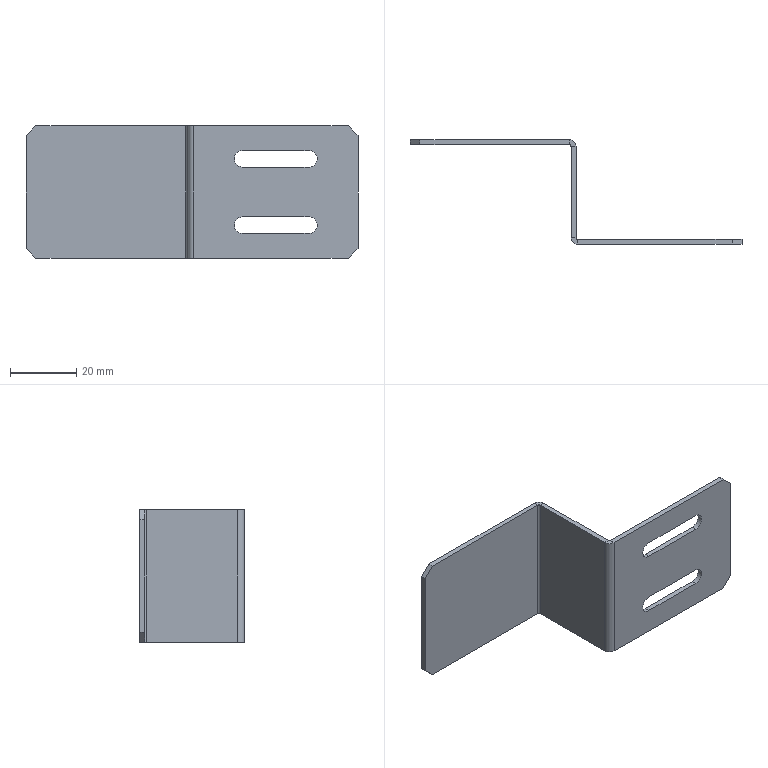Part | SolidWorks | features Chamfer 1, Cut 1, FlatPattern 1, SMBaseFlange 1, SheetMetal 1 | 1 solid | 34 faces | box 100 x 31.5 x 40 mm | volume 7350 mm3 | plane 26 | cylinder 8 | commonest cylinder face diameters 5 x4 1 x2 4 x2
STEP:
#1=CARTESIAN_POINT('',(0.,13.,20.));
#2=VERTEX_POINT('',#1);
#3=CARTESIAN_POINT('',(-1.5,13.,20.));
#4=VERTEX_POINT('',#3);
#5=CARTESIAN_POINT('',(0.,13.,20.));
#6=DIRECTION('',(-1.,0.,0.));
#7=VECTOR('',#6,1000.);
#8=LINE('',#5,#7);
#9=EDGE_CURVE('',#2,#4,#8,.T.);
#10=ORIENTED_EDGE('',*,*,#9,.F.);
#11=CARTESIAN_POINT('',(-2.,15.,20.));
#12=VERTEX_POINT('',#11);
#13=CARTESIAN_POINT('',(-2.,13.,20.));
#14=DIRECTION('',(0.,0.,-1.));
#15=DIRECTION('',(1.,0.,0.));
#16=AXIS2_PLACEMENT_3D('',#13,#14,#15);
#17=CIRCLE('',#16,2.);
#18=EDGE_CURVE('',#12,#2,#17,.T.);
#19=ORIENTED_EDGE('',*,*,#18,.F.);
#20=CARTESIAN_POINT('',(-2.,13.5,20.));
#21=VERTEX_POINT('',#20);
#22=CARTESIAN_POINT('',(-2.,13.5,20.));
#23=DIRECTION('',(0.,1.,0.));
#24=VECTOR('',#23,1000.);
#25=LINE('',#22,#24);
#26=EDGE_CURVE('',#21,#12,#25,.T.);
#27=ORIENTED_EDGE('',*,*,#26,.F.);
#28=CARTESIAN_POINT('',(-2.,13.,20.));
#29=DIRECTION('',(0.,0.,-1.));
#30=DIRECTION('',(1.,0.,0.));
#31=AXIS2_PLACEMENT_3D('',#28,#29,#30);
#32=CIRCLE('',#31,0.5);
#33=EDGE_CURVE('',#21,#4,#32,.T.);
#34=ORIENTED_EDGE('',*,*,#33,.T.);
#35=EDGE_LOOP('',(#10,#19,#27,#34));
#36=FACE_OUTER_BOUND('',#35,.T.);
#37=CARTESIAN_POINT('',(0.,13.,20.));
#38=DIRECTION('',(0.,0.,1.));
#39=DIRECTION('',(1.,0.,0.));
#40=AXIS2_PLACEMENT_3D('',#37,#38,#39);
#41=PLANE('',#40);
#42=ADVANCED_FACE('',(#36),#41,.T.);
#43=CARTESIAN_POINT('',(0.,-14.5,20.));
#44=VERTEX_POINT('',#43);
#45=CARTESIAN_POINT('',(0.,15.,20.));
#46=DIRECTION('',(0.,-1.,0.));
#47=VECTOR('',#46,1000.);
#48=LINE('',#45,#47);
#49=EDGE_CURVE('',#2,#44,#48,.T.);
#50=ORIENTED_EDGE('',*,*,#49,.F.);
#51=ORIENTED_EDGE('',*,*,#9,.T.);
#52=CARTESIAN_POINT('',(-1.5,-14.5,20.));
#53=VERTEX_POINT('',#52);
#54=CARTESIAN_POINT('',(-1.5,15.,20.));
#55=DIRECTION('',(0.,-1.,0.));
#56=VECTOR('',#55,1000.);
#57=LINE('',#54,#56);
#58=EDGE_CURVE('',#4,#53,#57,.T.);
#59=ORIENTED_EDGE('',*,*,#58,.T.);
#60=CARTESIAN_POINT('',(-1.5,-14.5,20.));
#61=DIRECTION('',(1.,0.,0.));
#62=VECTOR('',#61,1000.);
#63=LINE('',#60,#62);
#64=EDGE_CURVE('',#53,#44,#63,.T.);
#65=ORIENTED_EDGE('',*,*,#64,.T.);
#66=EDGE_LOOP('',(#50,#51,#59,#65));
#67=FACE_OUTER_BOUND('',#66,.T.);
#68=CARTESIAN_POINT('',(-2.,13.5,20.));
#69=DIRECTION('',(0.,0.,1.));
#70=DIRECTION('',(1.,0.,0.));
#71=AXIS2_PLACEMENT_3D('',#68,#69,#70);
#72=PLANE('',#71);
#73=ADVANCED_FACE('',(#67),#72,.T.);
#74=CARTESIAN_POINT('',(-2.,15.,-20.));
#75=VERTEX_POINT('',#74);
#76=CARTESIAN_POINT('',(-2.,13.5,-20.));
#77=VERTEX_POINT('',#76);
#78=CARTESIAN_POINT('',(-2.,15.,-20.));
#79=DIRECTION('',(0.,-1.,0.));
#80=VECTOR('',#79,1000.);
#81=LINE('',#78,#80);
#82=EDGE_CURVE('',#75,#77,#81,.T.);
#83=ORIENTED_EDGE('',*,*,#82,.F.);
#84=CARTESIAN_POINT('',(0.,13.,-20.));
#85=VERTEX_POINT('',#84);
#86=CARTESIAN_POINT('',(-2.,13.,-20.));
#87=DIRECTION('',(0.,0.,-1.));
#88=DIRECTION('',(1.,0.,0.));
#89=AXIS2_PLACEMENT_3D('',#86,#87,#88);
#90=CIRCLE('',#89,2.);
#91=EDGE_CURVE('',#75,#85,#90,.T.);
#92=ORIENTED_EDGE('',*,*,#91,.T.);
#93=CARTESIAN_POINT('',(-1.5,13.,-20.));
#94=VERTEX_POINT('',#93);
#95=CARTESIAN_POINT('',(-1.5,13.,-20.));
#96=DIRECTION('',(1.,0.,0.));
#97=VECTOR('',#96,1000.);
#98=LINE('',#95,#97);
#99=EDGE_CURVE('',#94,#85,#98,.T.);
#100=ORIENTED_EDGE('',*,*,#99,.F.);
#101=CARTESIAN_POINT('',(-2.,13.,-20.));
#102=DIRECTION('',(0.,0.,-1.));
#103=DIRECTION('',(1.,0.,0.));
#104=AXIS2_PLACEMENT_3D('',#101,#102,#103);
#105=CIRCLE('',#104,0.5);
#106=EDGE_CURVE('',#77,#94,#105,.T.);
#107=ORIENTED_EDGE('',*,*,#106,.F.);
#108=EDGE_LOOP('',(#83,#92,#100,#107));
#109=FACE_OUTER_BOUND('',#108,.T.);
#110=CARTESIAN_POINT('',(-2.,15.,-20.));
#111=DIRECTION('',(0.,0.,-1.));
#112=DIRECTION('',(-1.,0.,0.));
#113=AXIS2_PLACEMENT_3D('',#110,#111,#112);
#114=PLANE('',#113);
#115=ADVANCED_FACE('',(#109),#114,.T.);
#116=CARTESIAN_POINT('',(-47.,13.5,-20.));
#117=VERTEX_POINT('',#116);
#118=CARTESIAN_POINT('',(-50.,13.5,-20.));
#119=DIRECTION('',(1.,0.,0.));
#120=VECTOR('',#119,1000.);
#121=LINE('',#118,#120);
#122=EDGE_CURVE('',#117,#77,#121,.T.);
#123=ORIENTED_EDGE('',*,*,#122,.F.);
#124=CARTESIAN_POINT('',(-47.,15.,-20.));
#125=VERTEX_POINT('',#124);
#126=CARTESIAN_POINT('',(-47.,13.,-20.));
#127=DIRECTION('',(0.,1.,0.));
#128=VECTOR('',#127,1000.);
#129=LINE('',#126,#128);
#130=EDGE_CURVE('',#117,#125,#129,.T.);
#131=ORIENTED_EDGE('',*,*,#130,.T.);
#132=CARTESIAN_POINT('',(-50.,15.,-20.));
#133=DIRECTION('',(1.,0.,0.));
#134=VECTOR('',#133,1000.);
#135=LINE('',#132,#134);
#136=EDGE_CURVE('',#125,#75,#135,.T.);
#137=ORIENTED_EDGE('',*,*,#136,.T.);
#138=ORIENTED_EDGE('',*,*,#82,.T.);
#139=EDGE_LOOP('',(#123,#131,#137,#138));
#140=FACE_OUTER_BOUND('',#139,.T.);
#141=CARTESIAN_POINT('',(-1.5,13.,-20.));
#142=DIRECTION('',(0.,0.,-1.));
#143=DIRECTION('',(-1.,0.,0.));
#144=AXIS2_PLACEMENT_3D('',#141,#142,#143);
#145=PLANE('',#144);
#146=ADVANCED_FACE('',(#140),#145,.T.);
#147=CARTESIAN_POINT('',(0.5,-15.,20.));
#148=VERTEX_POINT('',#147);
#149=CARTESIAN_POINT('',(0.5,-16.5,20.));
#150=VERTEX_POINT('',#149);
#151=CARTESIAN_POINT('',(0.5,-15.,20.));
#152=DIRECTION('',(0.,-1.,0.));
#153=VECTOR('',#152,1000.);
#154=LINE('',#151,#153);
#155=EDGE_CURVE('',#148,#150,#154,.T.);
#156=ORIENTED_EDGE('',*,*,#155,.F.);
#157=CARTESIAN_POINT('',(0.5,-14.5,20.));
#158=DIRECTION('',(0.,0.,1.));
#159=DIRECTION('',(-1.,0.,0.));
#160=AXIS2_PLACEMENT_3D('',#157,#158,#159);
#161=CIRCLE('',#160,0.5);
#162=EDGE_CURVE('',#44,#148,#161,.T.);
#163=ORIENTED_EDGE('',*,*,#162,.F.);
#164=ORIENTED_EDGE('',*,*,#64,.F.);
#165=CARTESIAN_POINT('',(0.5,-14.5,20.));
#166=DIRECTION('',(0.,0.,1.));
#167=DIRECTION('',(1.,0.,0.));
#168=AXIS2_PLACEMENT_3D('',#165,#166,#167);
#169=CIRCLE('',#168,2.);
#170=EDGE_CURVE('',#53,#150,#169,.T.);
#171=ORIENTED_EDGE('',*,*,#170,.T.);
#172=EDGE_LOOP('',(#156,#163,#164,#171));
#173=FACE_OUTER_BOUND('',#172,.T.);
#174=CARTESIAN_POINT('',(0.5,-15.,20.));
#175=DIRECTION('',(0.,0.,1.));
#176=DIRECTION('',(1.,0.,0.));
#177=AXIS2_PLACEMENT_3D('',#174,#175,#176);
#178=PLANE('',#177);
#179=ADVANCED_FACE('',(#173),#178,.T.);
#180=CARTESIAN_POINT('',(47.,-16.5,20.));
#181=VERTEX_POINT('',#180);
#182=CARTESIAN_POINT('',(0.,-16.5,20.));
#183=DIRECTION('',(1.,0.,0.));
#184=VECTOR('',#183,1000.);
#185=LINE('',#182,#184);
#186=EDGE_CURVE('',#150,#181,#185,.T.);
#187=ORIENTED_EDGE('',*,*,#186,.T.);
#188=CARTESIAN_POINT('',(47.,-15.,20.));
#189=VERTEX_POINT('',#188);
#190=CARTESIAN_POINT('',(47.,-14.5,20.));
#191=DIRECTION('',(0.,1.,0.));
#192=VECTOR('',#191,1000.);
#193=LINE('',#190,#192);
#194=EDGE_CURVE('',#181,#189,#193,.T.);
#195=ORIENTED_EDGE('',*,*,#194,.T.);
#196=CARTESIAN_POINT('',(0.,-15.,20.));
#197=DIRECTION('',(1.,0.,0.));
#198=VECTOR('',#197,1000.);
#199=LINE('',#196,#198);
#200=EDGE_CURVE('',#148,#189,#199,.T.);
#201=ORIENTED_EDGE('',*,*,#200,.F.);
#202=ORIENTED_EDGE('',*,*,#155,.T.);
#203=EDGE_LOOP('',(#187,#195,#201,#202));
#204=FACE_OUTER_BOUND('',#203,.T.);
#205=CARTESIAN_POINT('',(-1.5,-14.5,20.));
#206=DIRECTION('',(0.,0.,1.));
#207=DIRECTION('',(1.,0.,0.));
#208=AXIS2_PLACEMENT_3D('',#205,#206,#207);
#209=PLANE('',#208);
#210=ADVANCED_FACE('',(#204),#209,.T.);
#211=CARTESIAN_POINT('',(0.,-14.5,-20.));
#212=VERTEX_POINT('',#211);
#213=CARTESIAN_POINT('',(-1.5,-14.5,-20.));
#214=VERTEX_POINT('',#213);
#215=CARTESIAN_POINT('',(0.,-14.5,-20.));
#216=DIRECTION('',(-1.,0.,0.));
#217=VECTOR('',#216,1000.);
#218=LINE('',#215,#217);
#219=EDGE_CURVE('',#212,#214,#218,.T.);
#220=ORIENTED_EDGE('',*,*,#219,.F.);
#221=CARTESIAN_POINT('',(0.5,-15.,-20.));
#222=VERTEX_POINT('',#221);
#223=CARTESIAN_POINT('',(0.5,-14.5,-20.));
#224=DIRECTION('',(0.,0.,1.));
#225=DIRECTION('',(-1.,0.,0.));
#226=AXIS2_PLACEMENT_3D('',#223,#224,#225);
#227=CIRCLE('',#226,0.5);
#228=EDGE_CURVE('',#212,#222,#227,.T.);
#229=ORIENTED_EDGE('',*,*,#228,.T.);
#230=CARTESIAN_POINT('',(0.5,-16.5,-20.));
#231=VERTEX_POINT('',#230);
#232=CARTESIAN_POINT('',(0.5,-16.5,-20.));
#233=DIRECTION('',(0.,1.,0.));
#234=VECTOR('',#233,1000.);
#235=LINE('',#232,#234);
#236=EDGE_CURVE('',#231,#222,#235,.T.);
#237=ORIENTED_EDGE('',*,*,#236,.F.);
#238=CARTESIAN_POINT('',(0.5,-14.5,-20.));
#239=DIRECTION('',(0.,0.,1.));
#240=DIRECTION('',(1.,0.,0.));
#241=AXIS2_PLACEMENT_3D('',#238,#239,#240);
#242=CIRCLE('',#241,2.);
#243=EDGE_CURVE('',#214,#231,#242,.T.);
#244=ORIENTED_EDGE('',*,*,#243,.F.);
#245=EDGE_LOOP('',(#220,#229,#237,#244));
#246=FACE_OUTER_BOUND('',#245,.T.);
#247=CARTESIAN_POINT('',(0.,-14.5,-20.));
#248=DIRECTION('',(0.,0.,-1.));
#249=DIRECTION('',(-1.,0.,0.));
#250=AXIS2_PLACEMENT_3D('',#247,#248,#249);
#251=PLANE('',#250);
#252=ADVANCED_FACE('',(#246),#251,.T.);
#253=CARTESIAN_POINT('',(0.,15.,-20.));
#254=DIRECTION('',(0.,-1.,0.));
#255=VECTOR('',#254,1000.);
#256=LINE('',#253,#255);
#257=EDGE_CURVE('',#85,#212,#256,.T.);
#258=ORIENTED_EDGE('',*,*,#257,.T.);
#259=ORIENTED_EDGE('',*,*,#219,.T.);
#260=CARTESIAN_POINT('',(-1.5,15.,-20.));
#261=DIRECTION('',(0.,-1.,0.));
#262=VECTOR('',#261,1000.);
#263=LINE('',#260,#262);
#264=EDGE_CURVE('',#94,#214,#263,.T.);
#265=ORIENTED_EDGE('',*,*,#264,.F.);
#266=ORIENTED_EDGE('',*,*,#99,.T.);
#267=EDGE_LOOP('',(#258,#259,#265,#266));
#268=FACE_OUTER_BOUND('',#267,.T.);
#269=CARTESIAN_POINT('',(0.5,-16.5,-20.));
#270=DIRECTION('',(0.,0.,-1.));
#271=DIRECTION('',(-1.,0.,0.));
#272=AXIS2_PLACEMENT_3D('',#269,#270,#271);
#273=PLANE('',#272);
#274=ADVANCED_FACE('',(#268),#273,.T.);
#275=CARTESIAN_POINT('',(35.25,-16.5,-12.5));
#276=VERTEX_POINT('',#275);
#277=CARTESIAN_POINT('',(15.25,-16.5,-12.5));
#278=VERTEX_POINT('',#277);
#279=CARTESIAN_POINT('',(15.25,-16.5,-12.5));
#280=DIRECTION('',(-1.,0.,0.));
#281=VECTOR('',#280,1000.);
#282=LINE('',#279,#281);
#283=EDGE_CURVE('',#276,#278,#282,.T.);
#284=ORIENTED_EDGE('',*,*,#283,.T.);
#285=CARTESIAN_POINT('',(15.25,-16.5,-7.5));
#286=VERTEX_POINT('',#285);
#287=CARTESIAN_POINT('',(15.25,-16.5,-10.));
#288=DIRECTION('',(0.,1.,0.));
#289=DIRECTION('',(0.,0.,1.));
#290=AXIS2_PLACEMENT_3D('',#287,#288,#289);
#291=CIRCLE('',#290,2.5);
#292=EDGE_CURVE('',#278,#286,#291,.T.);
#293=ORIENTED_EDGE('',*,*,#292,.T.);
#294=CARTESIAN_POINT('',(35.25,-16.5,-7.5));
#295=VERTEX_POINT('',#294);
#296=CARTESIAN_POINT('',(15.25,-16.5,-7.5));
#297=DIRECTION('',(1.,0.,0.));
#298=VECTOR('',#297,1000.);
#299=LINE('',#296,#298);
#300=EDGE_CURVE('',#286,#295,#299,.T.);
#301=ORIENTED_EDGE('',*,*,#300,.T.);
#302=CARTESIAN_POINT('',(35.25,-16.5,-10.));
#303=DIRECTION('',(0.,1.,0.));
#304=DIRECTION('',(0.,0.,1.));
#305=AXIS2_PLACEMENT_3D('',#302,#303,#304);
#306=CIRCLE('',#305,2.5);
#307=EDGE_CURVE('',#295,#276,#306,.T.);
#308=ORIENTED_EDGE('',*,*,#307,.T.);
#309=EDGE_LOOP('',(#284,#293,#301,#308));
#310=FACE_BOUND('',#309,.T.);
#311=CARTESIAN_POINT('',(35.25,-16.5,7.5));
#312=VERTEX_POINT('',#311);
#313=CARTESIAN_POINT('',(15.25,-16.5,7.5));
#314=VERTEX_POINT('',#313);
#315=CARTESIAN_POINT('',(15.25,-16.5,7.5));
#316=DIRECTION('',(-1.,0.,0.));
#317=VECTOR('',#316,1000.);
#318=LINE('',#315,#317);
#319=EDGE_CURVE('',#312,#314,#318,.T.);
#320=ORIENTED_EDGE('',*,*,#319,.T.);
#321=CARTESIAN_POINT('',(15.25,-16.5,12.5));
#322=VERTEX_POINT('',#321);
#323=CARTESIAN_POINT('',(15.25,-16.5,10.));
#324=DIRECTION('',(0.,1.,0.));
#325=DIRECTION('',(0.,0.,1.));
#326=AXIS2_PLACEMENT_3D('',#323,#324,#325);
#327=CIRCLE('',#326,2.5);
#328=EDGE_CURVE('',#314,#322,#327,.T.);
#329=ORIENTED_EDGE('',*,*,#328,.T.);
#330=CARTESIAN_POINT('',(35.25,-16.5,12.5));
#331=VERTEX_POINT('',#330);
#332=CARTESIAN_POINT('',(15.25,-16.5,12.5));
#333=DIRECTION('',(1.,0.,0.));
#334=VECTOR('',#333,1000.);
#335=LINE('',#332,#334);
#336=EDGE_CURVE('',#322,#331,#335,.T.);
#337=ORIENTED_EDGE('',*,*,#336,.T.);
#338=CARTESIAN_POINT('',(35.25,-16.5,10.));
#339=DIRECTION('',(0.,1.,0.));
#340=DIRECTION('',(0.,0.,1.));
#341=AXIS2_PLACEMENT_3D('',#338,#339,#340);
#342=CIRCLE('',#341,2.5);
#343=EDGE_CURVE('',#331,#312,#342,.T.);
#344=ORIENTED_EDGE('',*,*,#343,.T.);
#345=EDGE_LOOP('',(#320,#329,#337,#344));
#346=FACE_BOUND('',#345,.T.);
#347=CARTESIAN_POINT('',(47.,-16.5,-20.));
#348=VERTEX_POINT('',#347);
#349=CARTESIAN_POINT('',(0.,-16.5,-20.));
#350=DIRECTION('',(1.,0.,0.));
#351=VECTOR('',#350,1000.);
#352=LINE('',#349,#351);
#353=EDGE_CURVE('',#231,#348,#352,.T.);
#354=ORIENTED_EDGE('',*,*,#353,.T.);
#355=CARTESIAN_POINT('',(50.,-16.5,-17.));
#356=VERTEX_POINT('',#355);
#357=CARTESIAN_POINT('',(47.,-16.5,-20.));
#358=DIRECTION('',(0.7071,0.,0.7071));
#359=VECTOR('',#358,1000.);
#360=LINE('',#357,#359);
#361=EDGE_CURVE('',#348,#356,#360,.T.);
#362=ORIENTED_EDGE('',*,*,#361,.T.);
#363=CARTESIAN_POINT('',(50.,-16.5,17.));
#364=VERTEX_POINT('',#363);
#365=CARTESIAN_POINT('',(50.,-16.5,20.));
#366=DIRECTION('',(0.,0.,-1.));
#367=VECTOR('',#366,1000.);
#368=LINE('',#365,#367);
#369=EDGE_CURVE('',#364,#356,#368,.T.);
#370=ORIENTED_EDGE('',*,*,#369,.F.);
#371=CARTESIAN_POINT('',(50.,-16.5,17.));
#372=DIRECTION('',(-0.7071,0.,0.7071));
#373=VECTOR('',#372,1000.);
#374=LINE('',#371,#373);
#375=EDGE_CURVE('',#364,#181,#374,.T.);
#376=ORIENTED_EDGE('',*,*,#375,.T.);
#377=ORIENTED_EDGE('',*,*,#186,.F.);
#378=CARTESIAN_POINT('',(0.5,-16.5,20.));
#379=DIRECTION('',(0.,0.,-1.));
#380=VECTOR('',#379,1000.);
#381=LINE('',#378,#380);
#382=EDGE_CURVE('',#150,#231,#381,.T.);
#383=ORIENTED_EDGE('',*,*,#382,.T.);
#384=EDGE_LOOP('',(#354,#362,#370,#376,#377,#383));
#385=FACE_OUTER_BOUND('',#384,.T.);
#386=CARTESIAN_POINT('',(0.,-16.5,20.));
#387=DIRECTION('',(0.,1.,0.));
#388=DIRECTION('',(0.,0.,1.));
#389=AXIS2_PLACEMENT_3D('',#386,#387,#388);
#390=PLANE('',#389);
#391=ADVANCED_FACE('',(#310,#346,#385),#390,.F.);
#392=ORIENTED_EDGE('',*,*,#369,.T.);
#393=CARTESIAN_POINT('',(50.,-15.,-17.));
#394=VERTEX_POINT('',#393);
#395=CARTESIAN_POINT('',(50.,-15.,-17.));
#396=DIRECTION('',(0.,1.,0.));
#397=VECTOR('',#396,1000.);
#398=LINE('',#395,#397);
#399=EDGE_CURVE('',#356,#394,#398,.T.);
#400=ORIENTED_EDGE('',*,*,#399,.T.);
#401=CARTESIAN_POINT('',(50.,-15.,17.));
#402=VERTEX_POINT('',#401);
#403=CARTESIAN_POINT('',(50.,-15.,20.));
#404=DIRECTION('',(0.,0.,-1.));
#405=VECTOR('',#404,1000.);
#406=LINE('',#403,#405);
#407=EDGE_CURVE('',#402,#394,#406,.T.);
#408=ORIENTED_EDGE('',*,*,#407,.F.);
#409=CARTESIAN_POINT('',(50.,-15.,17.));
#410=DIRECTION('',(0.,-1.,0.));
#411=VECTOR('',#410,1000.);
#412=LINE('',#409,#411);
#413=EDGE_CURVE('',#402,#364,#412,.T.);
#414=ORIENTED_EDGE('',*,*,#413,.T.);
#415=EDGE_LOOP('',(#392,#400,#408,#414));
#416=FACE_OUTER_BOUND('',#415,.T.);
#417=CARTESIAN_POINT('',(50.,-15.,20.));
#418=DIRECTION('',(1.,0.,0.));
#419=DIRECTION('',(0.,0.,-1.));
#420=AXIS2_PLACEMENT_3D('',#417,#418,#419);
#421=PLANE('',#420);
#422=ADVANCED_FACE('',(#416),#421,.T.);
#423=CARTESIAN_POINT('',(15.25,-15.,-12.5));
#424=VERTEX_POINT('',#423);
#425=CARTESIAN_POINT('',(15.25,-15.,-7.5));
#426=VERTEX_POINT('',#425);
#427=CARTESIAN_POINT('',(15.25,-15.,-10.));
#428=DIRECTION('',(0.,1.,0.));
#429=DIRECTION('',(0.,0.,1.));
#430=AXIS2_PLACEMENT_3D('',#427,#428,#429);
#431=CIRCLE('',#430,2.5);
#432=EDGE_CURVE('',#424,#426,#431,.T.);
#433=ORIENTED_EDGE('',*,*,#432,.F.);
#434=CARTESIAN_POINT('',(35.25,-15.,-12.5));
#435=VERTEX_POINT('',#434);
#436=CARTESIAN_POINT('',(15.25,-15.,-12.5));
#437=DIRECTION('',(-1.,0.,0.));
#438=VECTOR('',#437,1000.);
#439=LINE('',#436,#438);
#440=EDGE_CURVE('',#435,#424,#439,.T.);
#441=ORIENTED_EDGE('',*,*,#440,.F.);
#442=CARTESIAN_POINT('',(35.25,-15.,-7.5));
#443=VERTEX_POINT('',#442);
#444=CARTESIAN_POINT('',(35.25,-15.,-10.));
#445=DIRECTION('',(0.,1.,0.));
#446=DIRECTION('',(0.,0.,1.));
#447=AXIS2_PLACEMENT_3D('',#444,#445,#446);
#448=CIRCLE('',#447,2.5);
#449=EDGE_CURVE('',#443,#435,#448,.T.);
#450=ORIENTED_EDGE('',*,*,#449,.F.);
#451=CARTESIAN_POINT('',(15.25,-15.,-7.5));
#452=DIRECTION('',(1.,0.,0.));
#453=VECTOR('',#452,1000.);
#454=LINE('',#451,#453);
#455=EDGE_CURVE('',#426,#443,#454,.T.);
#456=ORIENTED_EDGE('',*,*,#455,.F.);
#457=EDGE_LOOP('',(#433,#441,#450,#456));
#458=FACE_BOUND('',#457,.T.);
#459=CARTESIAN_POINT('',(15.25,-15.,7.5));
#460=VERTEX_POINT('',#459);
#461=CARTESIAN_POINT('',(15.25,-15.,12.5));
#462=VERTEX_POINT('',#461);
#463=CARTESIAN_POINT('',(15.25,-15.,10.));
#464=DIRECTION('',(0.,1.,0.));
#465=DIRECTION('',(0.,0.,1.));
#466=AXIS2_PLACEMENT_3D('',#463,#464,#465);
#467=CIRCLE('',#466,2.5);
#468=EDGE_CURVE('',#460,#462,#467,.T.);
#469=ORIENTED_EDGE('',*,*,#468,.F.);
#470=CARTESIAN_POINT('',(35.25,-15.,7.5));
#471=VERTEX_POINT('',#470);
#472=CARTESIAN_POINT('',(15.25,-15.,7.5));
#473=DIRECTION('',(-1.,0.,0.));
#474=VECTOR('',#473,1000.);
#475=LINE('',#472,#474);
#476=EDGE_CURVE('',#471,#460,#475,.T.);
#477=ORIENTED_EDGE('',*,*,#476,.F.);
#478=CARTESIAN_POINT('',(35.25,-15.,12.5));
#479=VERTEX_POINT('',#478);
#480=CARTESIAN_POINT('',(35.25,-15.,10.));
#481=DIRECTION('',(0.,1.,0.));
#482=DIRECTION('',(0.,0.,1.));
#483=AXIS2_PLACEMENT_3D('',#480,#481,#482);
#484=CIRCLE('',#483,2.5);
#485=EDGE_CURVE('',#479,#471,#484,.T.);
#486=ORIENTED_EDGE('',*,*,#485,.F.);
#487=CARTESIAN_POINT('',(15.25,-15.,12.5));
#488=DIRECTION('',(1.,0.,0.));
#489=VECTOR('',#488,1000.);
#490=LINE('',#487,#489);
#491=EDGE_CURVE('',#462,#479,#490,.T.);
#492=ORIENTED_EDGE('',*,*,#491,.F.);
#493=EDGE_LOOP('',(#469,#477,#486,#492));
#494=FACE_BOUND('',#493,.T.);
#495=ORIENTED_EDGE('',*,*,#407,.T.);
#496=CARTESIAN_POINT('',(47.,-15.,-20.));
#497=VERTEX_POINT('',#496);
#498=CARTESIAN_POINT('',(43.5,-15.,-23.5));
#499=DIRECTION('',(-0.7071,0.,-0.7071));
#500=VECTOR('',#499,1000.);
#501=LINE('',#498,#500);
#502=EDGE_CURVE('',#394,#497,#501,.T.);
#503=ORIENTED_EDGE('',*,*,#502,.T.);
#504=CARTESIAN_POINT('',(0.,-15.,-20.));
#505=DIRECTION('',(1.,0.,0.));
#506=VECTOR('',#505,1000.);
#507=LINE('',#504,#506);
#508=EDGE_CURVE('',#222,#497,#507,.T.);
#509=ORIENTED_EDGE('',*,*,#508,.F.);
#510=CARTESIAN_POINT('',(0.5,-15.,20.));
#511=DIRECTION('',(0.,0.,-1.));
#512=VECTOR('',#511,1000.);
#513=LINE('',#510,#512);
#514=EDGE_CURVE('',#148,#222,#513,.T.);
#515=ORIENTED_EDGE('',*,*,#514,.F.);
#516=ORIENTED_EDGE('',*,*,#200,.T.);
#517=CARTESIAN_POINT('',(23.5,-15.,43.5));
#518=DIRECTION('',(0.7071,0.,-0.7071));
#519=VECTOR('',#518,1000.);
#520=LINE('',#517,#519);
#521=EDGE_CURVE('',#189,#402,#520,.T.);
#522=ORIENTED_EDGE('',*,*,#521,.T.);
#523=EDGE_LOOP('',(#495,#503,#509,#515,#516,#522));
#524=FACE_OUTER_BOUND('',#523,.T.);
#525=CARTESIAN_POINT('',(0.,-15.,20.));
#526=DIRECTION('',(0.,1.,0.));
#527=DIRECTION('',(0.,0.,1.));
#528=AXIS2_PLACEMENT_3D('',#525,#526,#527);
#529=PLANE('',#528);
#530=ADVANCED_FACE('',(#458,#494,#524),#529,.T.);
#531=ORIENTED_EDGE('',*,*,#228,.F.);
#532=CARTESIAN_POINT('',(0.,-14.5,20.));
#533=DIRECTION('',(0.,0.,-1.));
#534=VECTOR('',#533,1000.);
#535=LINE('',#532,#534);
#536=EDGE_CURVE('',#44,#212,#535,.T.);
#537=ORIENTED_EDGE('',*,*,#536,.F.);
#538=ORIENTED_EDGE('',*,*,#162,.T.);
#539=ORIENTED_EDGE('',*,*,#514,.T.);
#540=EDGE_LOOP('',(#531,#537,#538,#539));
#541=FACE_OUTER_BOUND('',#540,.T.);
#542=CARTESIAN_POINT('',(0.5,-14.5,20.));
#543=DIRECTION('',(0.,0.,-1.));
#544=DIRECTION('',(-1.,0.,0.));
#545=AXIS2_PLACEMENT_3D('',#542,#543,#544);
#546=CYLINDRICAL_SURFACE('',#545,0.5);
#547=ADVANCED_FACE('',(#541),#546,.F.);
#548=ORIENTED_EDGE('',*,*,#257,.F.);
#549=CARTESIAN_POINT('',(0.,13.,20.));
#550=DIRECTION('',(0.,0.,-1.));
#551=VECTOR('',#550,1000.);
#552=LINE('',#549,#551);
#553=EDGE_CURVE('',#2,#85,#552,.T.);
#554=ORIENTED_EDGE('',*,*,#553,.F.);
#555=ORIENTED_EDGE('',*,*,#49,.T.);
#556=ORIENTED_EDGE('',*,*,#536,.T.);
#557=EDGE_LOOP('',(#548,#554,#555,#556));
#558=FACE_OUTER_BOUND('',#557,.T.);
#559=CARTESIAN_POINT('',(0.,15.,20.));
#560=DIRECTION('',(1.,0.,0.));
#561=DIRECTION('',(0.,0.,-1.));
#562=AXIS2_PLACEMENT_3D('',#559,#560,#561);
#563=PLANE('',#562);
#564=ADVANCED_FACE('',(#558),#563,.T.);
#565=ORIENTED_EDGE('',*,*,#91,.F.);
#566=CARTESIAN_POINT('',(-2.,15.,20.));
#567=DIRECTION('',(0.,0.,-1.));
#568=VECTOR('',#567,1000.);
#569=LINE('',#566,#568);
#570=EDGE_CURVE('',#12,#75,#569,.T.);
#571=ORIENTED_EDGE('',*,*,#570,.F.);
#572=ORIENTED_EDGE('',*,*,#18,.T.);
#573=ORIENTED_EDGE('',*,*,#553,.T.);
#574=EDGE_LOOP('',(#565,#571,#572,#573));
#575=FACE_OUTER_BOUND('',#574,.T.);
#576=CARTESIAN_POINT('',(-2.,13.,20.));
#577=DIRECTION('',(0.,0.,-1.));
#578=DIRECTION('',(-1.,0.,0.));
#579=AXIS2_PLACEMENT_3D('',#576,#577,#578);
#580=CYLINDRICAL_SURFACE('',#579,2.);
#581=ADVANCED_FACE('',(#575),#580,.T.);
#582=ORIENTED_EDGE('',*,*,#136,.F.);
#583=CARTESIAN_POINT('',(-50.,15.,-17.));
#584=VERTEX_POINT('',#583);
#585=CARTESIAN_POINT('',(-68.5,15.,1.5));
#586=DIRECTION('',(-0.7071,0.,0.7071));
#587=VECTOR('',#586,1000.);
#588=LINE('',#585,#587);
#589=EDGE_CURVE('',#125,#584,#588,.T.);
#590=ORIENTED_EDGE('',*,*,#589,.T.);
#591=CARTESIAN_POINT('',(-50.,15.,17.));
#592=VERTEX_POINT('',#591);
#593=CARTESIAN_POINT('',(-50.,15.,20.));
#594=DIRECTION('',(0.,0.,-1.));
#595=VECTOR('',#594,1000.);
#596=LINE('',#593,#595);
#597=EDGE_CURVE('',#592,#584,#596,.T.);
#598=ORIENTED_EDGE('',*,*,#597,.F.);
#599=CARTESIAN_POINT('',(-47.,15.,20.));
#600=VERTEX_POINT('',#599);
#601=CARTESIAN_POINT('',(-48.5,15.,18.5));
#602=DIRECTION('',(0.7071,0.,0.7071));
#603=VECTOR('',#602,1000.);
#604=LINE('',#601,#603);
#605=EDGE_CURVE('',#592,#600,#604,.T.);
#606=ORIENTED_EDGE('',*,*,#605,.T.);
#607=CARTESIAN_POINT('',(-50.,15.,20.));
#608=DIRECTION('',(1.,0.,0.));
#609=VECTOR('',#608,1000.);
#610=LINE('',#607,#609);
#611=EDGE_CURVE('',#600,#12,#610,.T.);
#612=ORIENTED_EDGE('',*,*,#611,.T.);
#613=ORIENTED_EDGE('',*,*,#570,.T.);
#614=EDGE_LOOP('',(#582,#590,#598,#606,#612,#613));
#615=FACE_OUTER_BOUND('',#614,.T.);
#616=CARTESIAN_POINT('',(-50.,15.,20.));
#617=DIRECTION('',(0.,1.,0.));
#618=DIRECTION('',(0.,0.,1.));
#619=AXIS2_PLACEMENT_3D('',#616,#617,#618);
#620=PLANE('',#619);
#621=ADVANCED_FACE('',(#615),#620,.T.);
#622=ORIENTED_EDGE('',*,*,#597,.T.);
#623=CARTESIAN_POINT('',(-50.,13.5,-17.));
#624=VERTEX_POINT('',#623);
#625=CARTESIAN_POINT('',(-50.,13.5,-17.));
#626=DIRECTION('',(0.,-1.,0.));
#627=VECTOR('',#626,1000.);
#628=LINE('',#625,#627);
#629=EDGE_CURVE('',#584,#624,#628,.T.);
#630=ORIENTED_EDGE('',*,*,#629,.T.);
#631=CARTESIAN_POINT('',(-50.,13.5,17.));
#632=VERTEX_POINT('',#631);
#633=CARTESIAN_POINT('',(-50.,13.5,20.));
#634=DIRECTION('',(0.,0.,-1.));
#635=VECTOR('',#634,1000.);
#636=LINE('',#633,#635);
#637=EDGE_CURVE('',#632,#624,#636,.T.);
#638=ORIENTED_EDGE('',*,*,#637,.F.);
#639=CARTESIAN_POINT('',(-50.,15.,17.));
#640=DIRECTION('',(0.,1.,0.));
#641=VECTOR('',#640,1000.);
#642=LINE('',#639,#641);
#643=EDGE_CURVE('',#632,#592,#642,.T.);
#644=ORIENTED_EDGE('',*,*,#643,.T.);
#645=EDGE_LOOP('',(#622,#630,#638,#644));
#646=FACE_OUTER_BOUND('',#645,.T.);
#647=CARTESIAN_POINT('',(-50.,13.5,20.));
#648=DIRECTION('',(-1.,0.,0.));
#649=DIRECTION('',(0.,0.,1.));
#650=AXIS2_PLACEMENT_3D('',#647,#648,#649);
#651=PLANE('',#650);
#652=ADVANCED_FACE('',(#646),#651,.T.);
#653=ORIENTED_EDGE('',*,*,#637,.T.);
#654=CARTESIAN_POINT('',(-47.,13.5,-20.));
#655=DIRECTION('',(0.7071,0.,-0.7071));
#656=VECTOR('',#655,1000.);
#657=LINE('',#654,#656);
#658=EDGE_CURVE('',#624,#117,#657,.T.);
#659=ORIENTED_EDGE('',*,*,#658,.T.);
#660=ORIENTED_EDGE('',*,*,#122,.T.);
#661=CARTESIAN_POINT('',(-2.,13.5,20.));
#662=DIRECTION('',(0.,0.,-1.));
#663=VECTOR('',#662,1000.);
#664=LINE('',#661,#663);
#665=EDGE_CURVE('',#21,#77,#664,.T.);
#666=ORIENTED_EDGE('',*,*,#665,.F.);
#667=CARTESIAN_POINT('',(-47.,13.5,20.));
#668=VERTEX_POINT('',#667);
#669=CARTESIAN_POINT('',(-50.,13.5,20.));
#670=DIRECTION('',(1.,0.,0.));
#671=VECTOR('',#670,1000.);
#672=LINE('',#669,#671);
#673=EDGE_CURVE('',#668,#21,#672,.T.);
#674=ORIENTED_EDGE('',*,*,#673,.F.);
#675=CARTESIAN_POINT('',(-50.,13.5,17.));
#676=DIRECTION('',(-0.7071,0.,-0.7071));
#677=VECTOR('',#676,1000.);
#678=LINE('',#675,#677);
#679=EDGE_CURVE('',#668,#632,#678,.T.);
#680=ORIENTED_EDGE('',*,*,#679,.T.);
#681=EDGE_LOOP('',(#653,#659,#660,#666,#674,#680));
#682=FACE_OUTER_BOUND('',#681,.T.);
#683=CARTESIAN_POINT('',(-50.,13.5,20.));
#684=DIRECTION('',(0.,1.,0.));
#685=DIRECTION('',(0.,0.,1.));
#686=AXIS2_PLACEMENT_3D('',#683,#684,#685);
#687=PLANE('',#686);
#688=ADVANCED_FACE('',(#682),#687,.F.);
#689=ORIENTED_EDGE('',*,*,#106,.T.);
#690=CARTESIAN_POINT('',(-1.5,13.,20.));
#691=DIRECTION('',(0.,0.,-1.));
#692=VECTOR('',#691,1000.);
#693=LINE('',#690,#692);
#694=EDGE_CURVE('',#4,#94,#693,.T.);
#695=ORIENTED_EDGE('',*,*,#694,.F.);
#696=ORIENTED_EDGE('',*,*,#33,.F.);
#697=ORIENTED_EDGE('',*,*,#665,.T.);
#698=EDGE_LOOP('',(#689,#695,#696,#697));
#699=FACE_OUTER_BOUND('',#698,.T.);
#700=CARTESIAN_POINT('',(-2.,13.,20.));
#701=DIRECTION('',(0.,0.,-1.));
#702=DIRECTION('',(-1.,0.,0.));
#703=AXIS2_PLACEMENT_3D('',#700,#701,#702);
#704=CYLINDRICAL_SURFACE('',#703,0.5);
#705=ADVANCED_FACE('',(#699),#704,.F.);
#706=ORIENTED_EDGE('',*,*,#264,.T.);
#707=CARTESIAN_POINT('',(-1.5,-14.5,20.));
#708=DIRECTION('',(0.,0.,-1.));
#709=VECTOR('',#708,1000.);
#710=LINE('',#707,#709);
#711=EDGE_CURVE('',#53,#214,#710,.T.);
#712=ORIENTED_EDGE('',*,*,#711,.F.);
#713=ORIENTED_EDGE('',*,*,#58,.F.);
#714=ORIENTED_EDGE('',*,*,#694,.T.);
#715=EDGE_LOOP('',(#706,#712,#713,#714));
#716=FACE_OUTER_BOUND('',#715,.T.);
#717=CARTESIAN_POINT('',(-1.5,15.,20.));
#718=DIRECTION('',(1.,0.,0.));
#719=DIRECTION('',(0.,0.,-1.));
#720=AXIS2_PLACEMENT_3D('',#717,#718,#719);
#721=PLANE('',#720);
#722=ADVANCED_FACE('',(#716),#721,.F.);
#723=ORIENTED_EDGE('',*,*,#243,.T.);
#724=ORIENTED_EDGE('',*,*,#382,.F.);
#725=ORIENTED_EDGE('',*,*,#170,.F.);
#726=ORIENTED_EDGE('',*,*,#711,.T.);
#727=EDGE_LOOP('',(#723,#724,#725,#726));
#728=FACE_OUTER_BOUND('',#727,.T.);
#729=CARTESIAN_POINT('',(0.5,-14.5,20.));
#730=DIRECTION('',(0.,0.,-1.));
#731=DIRECTION('',(-1.,0.,0.));
#732=AXIS2_PLACEMENT_3D('',#729,#730,#731);
#733=CYLINDRICAL_SURFACE('',#732,2.);
#734=ADVANCED_FACE('',(#728),#733,.T.);
#735=ORIENTED_EDGE('',*,*,#611,.F.);
#736=CARTESIAN_POINT('',(-47.,13.5,20.));
#737=DIRECTION('',(0.,-1.,0.));
#738=VECTOR('',#737,1000.);
#739=LINE('',#736,#738);
#740=EDGE_CURVE('',#600,#668,#739,.T.);
#741=ORIENTED_EDGE('',*,*,#740,.T.);
#742=ORIENTED_EDGE('',*,*,#673,.T.);
#743=ORIENTED_EDGE('',*,*,#26,.T.);
#744=EDGE_LOOP('',(#735,#741,#742,#743));
#745=FACE_OUTER_BOUND('',#744,.T.);
#746=CARTESIAN_POINT('',(0.5,-14.5,20.));
#747=DIRECTION('',(0.,0.,-1.));
#748=DIRECTION('',(-1.,0.,0.));
#749=AXIS2_PLACEMENT_3D('',#746,#747,#748);
#750=PLANE('',#749);
#751=ADVANCED_FACE('',(#745),#750,.F.);
#752=ORIENTED_EDGE('',*,*,#508,.T.);
#753=CARTESIAN_POINT('',(47.,-14.5,-20.));
#754=DIRECTION('',(0.,-1.,0.));
#755=VECTOR('',#754,1000.);
#756=LINE('',#753,#755);
#757=EDGE_CURVE('',#497,#348,#756,.T.);
#758=ORIENTED_EDGE('',*,*,#757,.T.);
#759=ORIENTED_EDGE('',*,*,#353,.F.);
#760=ORIENTED_EDGE('',*,*,#236,.T.);
#761=EDGE_LOOP('',(#752,#758,#759,#760));
#762=FACE_OUTER_BOUND('',#761,.T.);
#763=CARTESIAN_POINT('',(0.5,-14.5,-20.));
#764=DIRECTION('',(0.,0.,-1.));
#765=DIRECTION('',(-1.,0.,0.));
#766=AXIS2_PLACEMENT_3D('',#763,#764,#765);
#767=PLANE('',#766);
#768=ADVANCED_FACE('',(#762),#767,.T.);
#769=ORIENTED_EDGE('',*,*,#468,.T.);
#770=CARTESIAN_POINT('',(15.25,-16.5,12.5));
#771=DIRECTION('',(0.,1.,0.));
#772=VECTOR('',#771,1000.);
#773=LINE('',#770,#772);
#774=EDGE_CURVE('',#322,#462,#773,.T.);
#775=ORIENTED_EDGE('',*,*,#774,.F.);
#776=ORIENTED_EDGE('',*,*,#328,.F.);
#777=CARTESIAN_POINT('',(15.25,-16.5,7.5));
#778=DIRECTION('',(0.,1.,0.));
#779=VECTOR('',#778,1000.);
#780=LINE('',#777,#779);
#781=EDGE_CURVE('',#314,#460,#780,.T.);
#782=ORIENTED_EDGE('',*,*,#781,.T.);
#783=EDGE_LOOP('',(#769,#775,#776,#782));
#784=FACE_OUTER_BOUND('',#783,.T.);
#785=CARTESIAN_POINT('',(15.25,-16.5,10.));
#786=DIRECTION('',(0.,1.,0.));
#787=DIRECTION('',(0.,0.,1.));
#788=AXIS2_PLACEMENT_3D('',#785,#786,#787);
#789=CYLINDRICAL_SURFACE('',#788,2.5);
#790=ADVANCED_FACE('',(#784),#789,.F.);
#791=ORIENTED_EDGE('',*,*,#476,.T.);
#792=ORIENTED_EDGE('',*,*,#781,.F.);
#793=ORIENTED_EDGE('',*,*,#319,.F.);
#794=CARTESIAN_POINT('',(35.25,-16.5,7.5));
#795=DIRECTION('',(0.,1.,0.));
#796=VECTOR('',#795,1000.);
#797=LINE('',#794,#796);
#798=EDGE_CURVE('',#312,#471,#797,.T.);
#799=ORIENTED_EDGE('',*,*,#798,.T.);
#800=EDGE_LOOP('',(#791,#792,#793,#799));
#801=FACE_OUTER_BOUND('',#800,.T.);
#802=CARTESIAN_POINT('',(15.25,-16.5,7.5));
#803=DIRECTION('',(0.,0.,-1.));
#804=DIRECTION('',(-1.,0.,0.));
#805=AXIS2_PLACEMENT_3D('',#802,#803,#804);
#806=PLANE('',#805);
#807=ADVANCED_FACE('',(#801),#806,.F.);
#808=ORIENTED_EDGE('',*,*,#485,.T.);
#809=ORIENTED_EDGE('',*,*,#798,.F.);
#810=ORIENTED_EDGE('',*,*,#343,.F.);
#811=CARTESIAN_POINT('',(35.25,-16.5,12.5));
#812=DIRECTION('',(0.,1.,0.));
#813=VECTOR('',#812,1000.);
#814=LINE('',#811,#813);
#815=EDGE_CURVE('',#331,#479,#814,.T.);
#816=ORIENTED_EDGE('',*,*,#815,.T.);
#817=EDGE_LOOP('',(#808,#809,#810,#816));
#818=FACE_OUTER_BOUND('',#817,.T.);
#819=CARTESIAN_POINT('',(35.25,-16.5,10.));
#820=DIRECTION('',(0.,1.,0.));
#821=DIRECTION('',(0.,0.,1.));
#822=AXIS2_PLACEMENT_3D('',#819,#820,#821);
#823=CYLINDRICAL_SURFACE('',#822,2.5);
#824=ADVANCED_FACE('',(#818),#823,.F.);
#825=ORIENTED_EDGE('',*,*,#491,.T.);
#826=ORIENTED_EDGE('',*,*,#815,.F.);
#827=ORIENTED_EDGE('',*,*,#336,.F.);
#828=ORIENTED_EDGE('',*,*,#774,.T.);
#829=EDGE_LOOP('',(#825,#826,#827,#828));
#830=FACE_OUTER_BOUND('',#829,.T.);
#831=CARTESIAN_POINT('',(15.25,-16.5,12.5));
#832=DIRECTION('',(0.,0.,1.));
#833=DIRECTION('',(1.,0.,0.));
#834=AXIS2_PLACEMENT_3D('',#831,#832,#833);
#835=PLANE('',#834);
#836=ADVANCED_FACE('',(#830),#835,.F.);
#837=ORIENTED_EDGE('',*,*,#432,.T.);
#838=CARTESIAN_POINT('',(15.25,-16.5,-7.5));
#839=DIRECTION('',(0.,1.,0.));
#840=VECTOR('',#839,1000.);
#841=LINE('',#838,#840);
#842=EDGE_CURVE('',#286,#426,#841,.T.);
#843=ORIENTED_EDGE('',*,*,#842,.F.);
#844=ORIENTED_EDGE('',*,*,#292,.F.);
#845=CARTESIAN_POINT('',(15.25,-16.5,-12.5));
#846=DIRECTION('',(0.,1.,0.));
#847=VECTOR('',#846,1000.);
#848=LINE('',#845,#847);
#849=EDGE_CURVE('',#278,#424,#848,.T.);
#850=ORIENTED_EDGE('',*,*,#849,.T.);
#851=EDGE_LOOP('',(#837,#843,#844,#850));
#852=FACE_OUTER_BOUND('',#851,.T.);
#853=CARTESIAN_POINT('',(15.25,-16.5,-10.));
#854=DIRECTION('',(0.,1.,0.));
#855=DIRECTION('',(0.,0.,1.));
#856=AXIS2_PLACEMENT_3D('',#853,#854,#855);
#857=CYLINDRICAL_SURFACE('',#856,2.5);
#858=ADVANCED_FACE('',(#852),#857,.F.);
#859=ORIENTED_EDGE('',*,*,#440,.T.);
#860=ORIENTED_EDGE('',*,*,#849,.F.);
#861=ORIENTED_EDGE('',*,*,#283,.F.);
#862=CARTESIAN_POINT('',(35.25,-16.5,-12.5));
#863=DIRECTION('',(0.,1.,0.));
#864=VECTOR('',#863,1000.);
#865=LINE('',#862,#864);
#866=EDGE_CURVE('',#276,#435,#865,.T.);
#867=ORIENTED_EDGE('',*,*,#866,.T.);
#868=EDGE_LOOP('',(#859,#860,#861,#867));
#869=FACE_OUTER_BOUND('',#868,.T.);
#870=CARTESIAN_POINT('',(15.25,-16.5,-12.5));
#871=DIRECTION('',(0.,0.,-1.));
#872=DIRECTION('',(-1.,0.,0.));
#873=AXIS2_PLACEMENT_3D('',#870,#871,#872);
#874=PLANE('',#873);
#875=ADVANCED_FACE('',(#869),#874,.F.);
#876=ORIENTED_EDGE('',*,*,#449,.T.);
#877=ORIENTED_EDGE('',*,*,#866,.F.);
#878=ORIENTED_EDGE('',*,*,#307,.F.);
#879=CARTESIAN_POINT('',(35.25,-16.5,-7.5));
#880=DIRECTION('',(0.,1.,0.));
#881=VECTOR('',#880,1000.);
#882=LINE('',#879,#881);
#883=EDGE_CURVE('',#295,#443,#882,.T.);
#884=ORIENTED_EDGE('',*,*,#883,.T.);
#885=EDGE_LOOP('',(#876,#877,#878,#884));
#886=FACE_OUTER_BOUND('',#885,.T.);
#887=CARTESIAN_POINT('',(35.25,-16.5,-10.));
#888=DIRECTION('',(0.,1.,0.));
#889=DIRECTION('',(0.,0.,1.));
#890=AXIS2_PLACEMENT_3D('',#887,#888,#889);
#891=CYLINDRICAL_SURFACE('',#890,2.5);
#892=ADVANCED_FACE('',(#886),#891,.F.);
#893=ORIENTED_EDGE('',*,*,#455,.T.);
#894=ORIENTED_EDGE('',*,*,#883,.F.);
#895=ORIENTED_EDGE('',*,*,#300,.F.);
#896=ORIENTED_EDGE('',*,*,#842,.T.);
#897=EDGE_LOOP('',(#893,#894,#895,#896));
#898=FACE_OUTER_BOUND('',#897,.T.);
#899=CARTESIAN_POINT('',(15.25,-16.5,-7.5));
#900=DIRECTION('',(0.,0.,1.));
#901=DIRECTION('',(1.,0.,0.));
#902=AXIS2_PLACEMENT_3D('',#899,#900,#901);
#903=PLANE('',#902);
#904=ADVANCED_FACE('',(#898),#903,.F.);
#905=ORIENTED_EDGE('',*,*,#658,.F.);
#906=ORIENTED_EDGE('',*,*,#629,.F.);
#907=ORIENTED_EDGE('',*,*,#589,.F.);
#908=ORIENTED_EDGE('',*,*,#130,.F.);
#909=EDGE_LOOP('',(#905,#906,#907,#908));
#910=FACE_OUTER_BOUND('',#909,.T.);
#911=CARTESIAN_POINT('',(-47.,13.,-20.));
#912=DIRECTION('',(0.7071,0.,0.7071));
#913=DIRECTION('',(0.,1.,0.));
#914=AXIS2_PLACEMENT_3D('',#911,#912,#913);
#915=PLANE('',#914);
#916=ADVANCED_FACE('',(#910),#915,.F.);
#917=ORIENTED_EDGE('',*,*,#679,.F.);
#918=ORIENTED_EDGE('',*,*,#740,.F.);
#919=ORIENTED_EDGE('',*,*,#605,.F.);
#920=ORIENTED_EDGE('',*,*,#643,.F.);
#921=EDGE_LOOP('',(#917,#918,#919,#920));
#922=FACE_OUTER_BOUND('',#921,.T.);
#923=CARTESIAN_POINT('',(-50.,13.5,17.));
#924=DIRECTION('',(-0.7071,0.,0.7071));
#925=DIRECTION('',(0.,-1.,0.));
#926=AXIS2_PLACEMENT_3D('',#923,#924,#925);
#927=PLANE('',#926);
#928=ADVANCED_FACE('',(#922),#927,.T.);
#929=ORIENTED_EDGE('',*,*,#502,.F.);
#930=ORIENTED_EDGE('',*,*,#399,.F.);
#931=ORIENTED_EDGE('',*,*,#361,.F.);
#932=ORIENTED_EDGE('',*,*,#757,.F.);
#933=EDGE_LOOP('',(#929,#930,#931,#932));
#934=FACE_OUTER_BOUND('',#933,.T.);
#935=CARTESIAN_POINT('',(47.,-14.5,-20.));
#936=DIRECTION('',(-0.7071,0.,0.7071));
#937=DIRECTION('',(0.,-1.,0.));
#938=AXIS2_PLACEMENT_3D('',#935,#936,#937);
#939=PLANE('',#938);
#940=ADVANCED_FACE('',(#934),#939,.F.);
#941=ORIENTED_EDGE('',*,*,#521,.F.);
#942=ORIENTED_EDGE('',*,*,#194,.F.);
#943=ORIENTED_EDGE('',*,*,#375,.F.);
#944=ORIENTED_EDGE('',*,*,#413,.F.);
#945=EDGE_LOOP('',(#941,#942,#943,#944));
#946=FACE_OUTER_BOUND('',#945,.T.);
#947=CARTESIAN_POINT('',(50.,-15.,17.));
#948=DIRECTION('',(-0.7071,0.,-0.7071));
#949=DIRECTION('',(0.,-1.,0.));
#950=AXIS2_PLACEMENT_3D('',#947,#948,#949);
#951=PLANE('',#950);
#952=ADVANCED_FACE('',(#946),#951,.F.);
#953=CLOSED_SHELL('',(#42,#73,#115,#146,#179,#210,#252,#274,#391,#422,#530,#547,#564,#581,#621,#652,#688,#705,#722,#734,#751,#768,#790,#807,#824,#836,#858,#875,#892,#904,#916,#928,#940,#952));
#954=MANIFOLD_SOLID_BREP('',#953);
#955=CARTESIAN_POINT('',(0.,0.,0.));
#956=DIRECTION('',(0.,0.,1.));
#957=DIRECTION('',(1.,0.,0.));
#958=AXIS2_PLACEMENT_3D('',#955,#956,#957);
#959=(LENGTH_UNIT()NAMED_UNIT(*)SI_UNIT(.MILLI.,.METRE.));
#960=UNCERTAINTY_MEASURE_WITH_UNIT(LENGTH_MEASURE(0.00001),#959,'','');
#961=(NAMED_UNIT(*)PLANE_ANGLE_UNIT()SI_UNIT($,.RADIAN.));
#962=(NAMED_UNIT(*)SI_UNIT($,.STERADIAN.)SOLID_ANGLE_UNIT());
#963=(GEOMETRIC_REPRESENTATION_CONTEXT(3)GLOBAL_UNCERTAINTY_ASSIGNED_CONTEXT((#960))GLOBAL_UNIT_ASSIGNED_CONTEXT((#959,#961,#962))REPRESENTATION_CONTEXT('',''));
#964=ADVANCED_BREP_SHAPE_REPRESENTATION('',(#954,#958),#963);